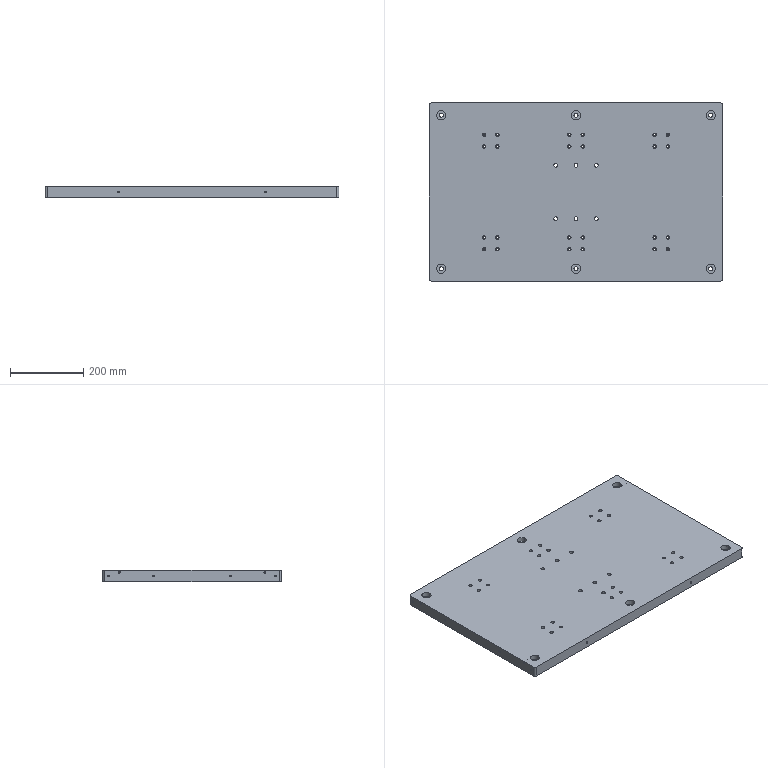NC program | Mastercam | posted with a generic post | part box 800 x 485 x 30 mm
Lines 1 to 982 of 7047:
%
O0000()
(MATERIAL - ALUMINUM MM - 2024)
( T20 | 20 FEM | H20 | XY STOCK TO LEAVE - .1 | Z STOCK TO LEAVE - .05 )
( T7 | 4 CHM | H7 )
( T1 | 11 DR | H1 )
( T15 | 5.5 DR | H15 )
( T14 | 10.5 DR | H14 )
( T5 | 5 FEM | H5 | XY STOCK TO LEAVE - -.01 | Z STOCK TO LEAVE - 0. )
( T9 | 10 FEM | H9 | XY STOCK TO LEAVE - .07 | Z STOCK TO LEAVE - .1 )
( T10 | 10 FEM | H10 | D10 | WEAR COMP | TOOL DIA. - 10. | XY STOCK TO LEAVE - -.02 | Z STOCK TO LEAVE - 0. )
( T18 | 5.1 DR | H18 )
N100 G21
N110 G0 G17 G40 G49 G80 G90
( ?X )
N120 T20 M6
N130 G0 G90 G54 X-415. Y252.6 A0. S5000 M3
N140 G43 H20 Z50. M8
N150 Z1.
N160 G1 Z-.998 F600.
N170 X-395. F4000.
N180 X395.
N190 X415.
N200 Z-1.997 F600.
N210 X395. F4000.
N220 X-395.
N230 X-415.
N240 Z-2.995 F600.
N250 X-395. F4000.
N260 X395.
N270 X415.
N280 Z-3.993 F600.
N290 X395. F4000.
N300 X-395.
N310 X-415.
N320 Z-4.992 F600.
N330 X-395. F4000.
N340 X395.
N350 X415.
N360 Z-5.99 F600.
N370 X395. F4000.
N380 X-395.
N390 X-415.
N400 Z-6.988 F600.
N410 X-395. F4000.
N420 X395.
N430 X415.
N440 Z-7.987 F600.
N450 X395. F4000.
N460 X-395.
N470 X-415.
N480 Z-8.985 F600.
N490 X-395. F4000.
N500 X395.
N510 X415.
N520 Z-9.983 F600.
N530 X395. F4000.
N540 X-395.
N550 X-415.
N560 Z-10.982 F600.
N570 X-395. F4000.
N580 X395.
N590 X415.
N600 Z-11.98 F600.
N610 X395. F4000.
N620 X-395.
N630 X-415.
N640 Z-12.978 F600.
N650 X-395. F4000.
N660 X395.
N670 X415.
N680 Z-13.977 F600.
N690 X395. F4000.
N700 X-395.
N710 X-415.
N720 Z-14.975 F600.
N730 X-395. F4000.
N740 X395.
N750 X415.
N760 Z-15.973 F600.
N770 X395. F4000.
N780 X-395.
N790 X-415.
N800 Z-16.972 F600.
N810 X-395. F4000.
N820 X395.
N830 X415.
N840 Z-17.97 F600.
N850 X395. F4000.
N860 X-395.
N870 X-415.
N880 Z-18.968 F600.
N890 X-395. F4000.
N900 X395.
N910 X415.
N920 Z-19.967 F600.
N930 X395. F4000.
N940 X-395.
N950 X-415.
N960 Z-20.965 F600.
N970 X-395. F4000.
N980 X395.
N990 X415.
N1000 Z-21.963 F600.
N1010 X395. F4000.
N1020 X-395.
N1030 X-415.
N1040 Z-22.962 F600.
N1050 X-395. F4000.
N1060 X395.
N1070 X415.
N1080 Z-23.96 F600.
N1090 X395. F4000.
N1100 X-395.
N1110 X-415.
N1120 Z-24.958 F600.
N1130 X-395. F4000.
N1140 X395.
N1150 X415.
N1160 Z-25.957 F600.
N1170 X395. F4000.
N1180 X-395.
N1190 X-415.
N1200 Z-26.955 F600.
N1210 X-395. F4000.
N1220 X395.
N1230 X415.
N1240 Z-27.953 F600.
N1250 X395. F4000.
N1260 X-395.
N1270 X-415.
N1280 Z-28.952 F600.
N1290 X-395. F4000.
N1300 X395.
N1310 X415.
N1320 Z-29.95 F600.
N1330 X395. F4000.
N1340 X-395.
N1350 X-415.
N1360 G0 Z50.
N1370 X415. Y-252.6
N1380 Z1.
N1390 G1 Z-.998 F600.
N1400 X395. F4000.
N1410 X-395.
N1420 X-415.
N1430 Z-1.997 F600.
N1440 X-395. F4000.
N1450 X395.
N1460 X415.
N1470 Z-2.995 F600.
N1480 X395. F4000.
N1490 X-395.
N1500 X-415.
N1510 Z-3.993 F600.
N1520 X-395. F4000.
N1530 X395.
N1540 X415.
N1550 Z-4.992 F600.
N1560 X395. F4000.
N1570 X-395.
N1580 X-415.
N1590 Z-5.99 F600.
N1600 X-395. F4000.
N1610 X395.
N1620 X415.
N1630 Z-6.988 F600.
N1640 X395. F4000.
N1650 X-395.
N1660 X-415.
N1670 Z-7.987 F600.
N1680 X-395. F4000.
N1690 X395.
N1700 X415.
N1710 Z-8.985 F600.
N1720 X395. F4000.
N1730 X-395.
N1740 X-415.
N1750 Z-9.983 F600.
N1760 X-395. F4000.
N1770 X395.
N1780 X415.
N1790 Z-10.982 F600.
N1800 X395. F4000.
N1810 X-395.
N1820 X-415.
N1830 Z-11.98 F600.
N1840 X-395. F4000.
N1850 X395.
N1860 X415.
N1870 Z-12.978 F600.
N1880 X395. F4000.
N1890 X-395.
N1900 X-415.
N1910 Z-13.977 F600.
N1920 X-395. F4000.
N1930 X395.
N1940 X415.
N1950 Z-14.975 F600.
N1960 X395. F4000.
N1970 X-395.
N1980 X-415.
N1990 Z-15.973 F600.
N2000 X-395. F4000.
N2010 X395.
N2020 X415.
N2030 Z-16.972 F600.
N2040 X395. F4000.
N2050 X-395.
N2060 X-415.
N2070 Z-17.97 F600.
N2080 X-395. F4000.
N2090 X395.
N2100 X415.
N2110 Z-18.968 F600.
N2120 X395. F4000.
N2130 X-395.
N2140 X-415.
N2150 Z-19.967 F600.
N2160 X-395. F4000.
N2170 X395.
N2180 X415.
N2190 Z-20.965 F600.
N2200 X395. F4000.
N2210 X-395.
N2220 X-415.
N2230 Z-21.963 F600.
N2240 X-395. F4000.
N2250 X395.
N2260 X415.
N2270 Z-22.962 F600.
N2280 X395. F4000.
N2290 X-395.
N2300 X-415.
N2310 Z-23.96 F600.
N2320 X-395. F4000.
N2330 X395.
N2340 X415.
N2350 Z-24.958 F600.
N2360 X395. F4000.
N2370 X-395.
N2380 X-415.
N2390 Z-25.957 F600.
N2400 X-395. F4000.
N2410 X395.
N2420 X415.
N2430 Z-26.955 F600.
N2440 X395. F4000.
N2450 X-395.
N2460 X-415.
N2470 Z-27.953 F600.
N2480 X-395. F4000.
N2490 X395.
N2500 X415.
N2510 Z-28.952 F600.
N2520 X395. F4000.
N2530 X-395.
N2540 X-415.
N2550 Z-29.95 F600.
N2560 X-395. F4000.
N2570 X395.
N2580 X415.
N2590 G0 Z50.
N2600 X-415. Y252.53
N2610 Z1.
N2620 G1 Z-29.95 F600.
N2630 X-395. F1000.
N2640 X395.
N2650 X415.
N2660 G0 Z50.
N2670 X-415. Y252.5
N2680 Z1.
N2690 G1 Z-29.95 F600.
N2700 X-395. F1000.
N2710 X395.
N2720 X415.
N2730 G0 Z50.
N2740 Y-252.53
N2750 Z1.
N2760 G1 Z-29.95 F600.
N2770 X395. F1000.
N2780 X-395.
N2790 X-415.
N2800 G0 Z50.
N2810 X415. Y-252.5
N2820 Z1.
N2830 G1 Z-29.95 F600.
N2840 X395. F1000.
N2850 X-395.
N2860 X-415.
N2870 G0 Z50.
N2880 M5
N2890 G91 G28 Z0. M9
N2900 A0.
N2910 M01
N2920 T7 M6
N2930 G0 G90 G17 G54 X-405. Y243.15 A0. S6500 M3
N2940 G43 H7 Z50. M8
N2950 Z1.
N2960 G1 Z-.75 F600.
N2970 X-395. F1000.
N2980 X395.
N2990 X405.
N3000 G0 Z50.
N3010 Y-243.15
N3020 Z1.
N3030 G1 Z-.75 F600.
N3040 X395. F1000.
N3050 X-395.
N3060 X-405.
N3070 G0 Z50.
N3080 M5
N3090 G91 G28 Z0. M9
N3100 A0.
N3110 M01
( CCL,CY )
M00
N3120 T20 M6
N3130 G0 G90 G17 G54 X-393. Y-256.6 A0. S5000 M3
N3140 G43 H20 Z50. M8
N3150 Z1.
N3160 G1 Z-.998 F600.
N3170 Y-254.6 F4000.
N3180 G3 X-395. Y-252.6 I-2. J0.
N3190 G2 X-410.1 Y-237.5 I0. J15.1
N3200 G1 Y237.5
N3210 G2 X-395. Y252.6 I15.1 J0.
N3220 G3 X-393. Y254.6 I0. J2.
N3230 G1 Y256.6
N3240 Z-1.997 F600.
N3250 Y254.6 F4000.
N3260 G2 X-395. Y252.6 I-2. J0.
N3270 G3 X-410.1 Y237.5 I0. J-15.1
N3280 G1 Y-237.5
N3290 G3 X-395. Y-252.6 I15.1 J0.
N3300 G2 X-393. Y-254.6 I0. J-2.
N3310 G1 Y-256.6
N3320 Z-2.995 F600.
N3330 Y-254.6 F4000.
N3340 G3 X-395. Y-252.6 I-2. J0.
N3350 G2 X-410.1 Y-237.5 I0. J15.1
N3360 G1 Y237.5
N3370 G2 X-395. Y252.6 I15.1 J0.
N3380 G3 X-393. Y254.6 I0. J2.
N3390 G1 Y256.6
N3400 Z-3.993 F600.
N3410 Y254.6 F4000.
N3420 G2 X-395. Y252.6 I-2. J0.
N3430 G3 X-410.1 Y237.5 I0. J-15.1
N3440 G1 Y-237.5
N3450 G3 X-395. Y-252.6 I15.1 J0.
N3460 G2 X-393. Y-254.6 I0. J-2.
N3470 G1 Y-256.6
N3480 Z-4.992 F600.
N3490 Y-254.6 F4000.
N3500 G3 X-395. Y-252.6 I-2. J0.
N3510 G2 X-410.1 Y-237.5 I0. J15.1
N3520 G1 Y237.5
N3530 G2 X-395. Y252.6 I15.1 J0.
N3540 G3 X-393. Y254.6 I0. J2.
N3550 G1 Y256.6
N3560 Z-5.99 F600.
N3570 Y254.6 F4000.
N3580 G2 X-395. Y252.6 I-2. J0.
N3590 G3 X-410.1 Y237.5 I0. J-15.1
N3600 G1 Y-237.5
N3610 G3 X-395. Y-252.6 I15.1 J0.
N3620 G2 X-393. Y-254.6 I0. J-2.
N3630 G1 Y-256.6
N3640 Z-6.988 F600.
N3650 Y-254.6 F4000.
N3660 G3 X-395. Y-252.6 I-2. J0.
N3670 G2 X-410.1 Y-237.5 I0. J15.1
N3680 G1 Y237.5
N3690 G2 X-395. Y252.6 I15.1 J0.
N3700 G3 X-393. Y254.6 I0. J2.
N3710 G1 Y256.6
N3720 Z-7.987 F600.
N3730 Y254.6 F4000.
N3740 G2 X-395. Y252.6 I-2. J0.
N3750 G3 X-410.1 Y237.5 I0. J-15.1
N3760 G1 Y-237.5
N3770 G3 X-395. Y-252.6 I15.1 J0.
N3780 G2 X-393. Y-254.6 I0. J-2.
N3790 G1 Y-256.6
N3800 Z-8.985 F600.
N3810 Y-254.6 F4000.
N3820 G3 X-395. Y-252.6 I-2. J0.
N3830 G2 X-410.1 Y-237.5 I0. J15.1
N3840 G1 Y237.5
N3850 G2 X-395. Y252.6 I15.1 J0.
N3860 G3 X-393. Y254.6 I0. J2.
N3870 G1 Y256.6
N3880 Z-9.983 F600.
N3890 Y254.6 F4000.
N3900 G2 X-395. Y252.6 I-2. J0.
N3910 G3 X-410.1 Y237.5 I0. J-15.1
N3920 G1 Y-237.5
N3930 G3 X-395. Y-252.6 I15.1 J0.
N3940 G2 X-393. Y-254.6 I0. J-2.
N3950 G1 Y-256.6
N3960 Z-10.982 F600.
N3970 Y-254.6 F4000.
N3980 G3 X-395. Y-252.6 I-2. J0.
N3990 G2 X-410.1 Y-237.5 I0. J15.1
N4000 G1 Y237.5
N4010 G2 X-395. Y252.6 I15.1 J0.
N4020 G3 X-393. Y254.6 I0. J2.
N4030 G1 Y256.6
N4040 Z-11.98 F600.
N4050 Y254.6 F4000.
N4060 G2 X-395. Y252.6 I-2. J0.
N4070 G3 X-410.1 Y237.5 I0. J-15.1
N4080 G1 Y-237.5
N4090 G3 X-395. Y-252.6 I15.1 J0.
N4100 G2 X-393. Y-254.6 I0. J-2.
N4110 G1 Y-256.6
N4120 Z-12.978 F600.
N4130 Y-254.6 F4000.
N4140 G3 X-395. Y-252.6 I-2. J0.
N4150 G2 X-410.1 Y-237.5 I0. J15.1
N4160 G1 Y237.5
N4170 G2 X-395. Y252.6 I15.1 J0.
N4180 G3 X-393. Y254.6 I0. J2.
N4190 G1 Y256.6
N4200 Z-13.977 F600.
N4210 Y254.6 F4000.
N4220 G2 X-395. Y252.6 I-2. J0.
N4230 G3 X-410.1 Y237.5 I0. J-15.1
N4240 G1 Y-237.5
N4250 G3 X-395. Y-252.6 I15.1 J0.
N4260 G2 X-393. Y-254.6 I0. J-2.
N4270 G1 Y-256.6
N4280 Z-14.975 F600.
N4290 Y-254.6 F4000.
N4300 G3 X-395. Y-252.6 I-2. J0.
N4310 G2 X-410.1 Y-237.5 I0. J15.1
N4320 G1 Y237.5
N4330 G2 X-395. Y252.6 I15.1 J0.
N4340 G3 X-393. Y254.6 I0. J2.
N4350 G1 Y256.6
N4360 Z-15.973 F600.
N4370 Y254.6 F4000.
N4380 G2 X-395. Y252.6 I-2. J0.
N4390 G3 X-410.1 Y237.5 I0. J-15.1
N4400 G1 Y-237.5
N4410 G3 X-395. Y-252.6 I15.1 J0.
N4420 G2 X-393. Y-254.6 I0. J-2.
N4430 G1 Y-256.6
N4440 Z-16.972 F600.
N4450 Y-254.6 F4000.
N4460 G3 X-395. Y-252.6 I-2. J0.
N4470 G2 X-410.1 Y-237.5 I0. J15.1
N4480 G1 Y237.5
N4490 G2 X-395. Y252.6 I15.1 J0.
N4500 G3 X-393. Y254.6 I0. J2.
N4510 G1 Y256.6
N4520 Z-17.97 F600.
N4530 Y254.6 F4000.
N4540 G2 X-395. Y252.6 I-2. J0.
N4550 G3 X-410.1 Y237.5 I0. J-15.1
N4560 G1 Y-237.5
N4570 G3 X-395. Y-252.6 I15.1 J0.
N4580 G2 X-393. Y-254.6 I0. J-2.
N4590 G1 Y-256.6
N4600 Z-18.968 F600.
N4610 Y-254.6 F4000.
N4620 G3 X-395. Y-252.6 I-2. J0.
N4630 G2 X-410.1 Y-237.5 I0. J15.1
N4640 G1 Y237.5
N4650 G2 X-395. Y252.6 I15.1 J0.
N4660 G3 X-393. Y254.6 I0. J2.
N4670 G1 Y256.6
N4680 Z-19.967 F600.
N4690 Y254.6 F4000.
N4700 G2 X-395. Y252.6 I-2. J0.
N4710 G3 X-410.1 Y237.5 I0. J-15.1
N4720 G1 Y-237.5
N4730 G3 X-395. Y-252.6 I15.1 J0.
N4740 G2 X-393. Y-254.6 I0. J-2.
N4750 G1 Y-256.6
N4760 Z-20.965 F600.
N4770 Y-254.6 F4000.
N4780 G3 X-395. Y-252.6 I-2. J0.
N4790 G2 X-410.1 Y-237.5 I0. J15.1
N4800 G1 Y237.5
N4810 G2 X-395. Y252.6 I15.1 J0.
N4820 G3 X-393. Y254.6 I0. J2.
N4830 G1 Y256.6
N4840 Z-21.963 F600.
N4850 Y254.6 F4000.
N4860 G2 X-395. Y252.6 I-2. J0.
N4870 G3 X-410.1 Y237.5 I0. J-15.1
N4880 G1 Y-237.5
N4890 G3 X-395. Y-252.6 I15.1 J0.
N4900 G2 X-393. Y-254.6 I0. J-2.
N4910 G1 Y-256.6
N4920 Z-22.962 F600.
N4930 Y-254.6 F4000.
N4940 G3 X-395. Y-252.6 I-2. J0.
N4950 G2 X-410.1 Y-237.5 I0. J15.1
N4960 G1 Y237.5
N4970 G2 X-395. Y252.6 I15.1 J0.
N4980 G3 X-393. Y254.6 I0. J2.
N4990 G1 Y256.6
N5000 Z-23.96 F600.
N5010 Y254.6 F4000.
N5020 G2 X-395. Y252.6 I-2. J0.
N5030 G3 X-410.1 Y237.5 I0. J-15.1
N5040 G1 Y-237.5
N5050 G3 X-395. Y-252.6 I15.1 J0.
N5060 G2 X-393. Y-254.6 I0. J-2.
N5070 G1 Y-256.6
N5080 Z-24.958 F600.
N5090 Y-254.6 F4000.
N5100 G3 X-395. Y-252.6 I-2. J0.
N5110 G2 X-410.1 Y-237.5 I0. J15.1
N5120 G1 Y237.5
N5130 G2 X-395. Y252.6 I15.1 J0.
N5140 G3 X-393. Y254.6 I0. J2.
N5150 G1 Y256.6
N5160 Z-25.957 F600.
N5170 Y254.6 F4000.
N5180 G2 X-395. Y252.6 I-2. J0.
N5190 G3 X-410.1 Y237.5 I0. J-15.1
N5200 G1 Y-237.5
N5210 G3 X-395. Y-252.6 I15.1 J0.
N5220 G2 X-393. Y-254.6 I0. J-2.
N5230 G1 Y-256.6
N5240 Z-26.955 F600.
N5250 Y-254.6 F4000.
N5260 G3 X-395. Y-252.6 I-2. J0.
N5270 G2 X-410.1 Y-237.5 I0. J15.1
N5280 G1 Y237.5
N5290 G2 X-395. Y252.6 I15.1 J0.
N5300 G3 X-393. Y254.6 I0. J2.
N5310 G1 Y256.6
N5320 Z-27.953 F600.
N5330 Y254.6 F4000.
N5340 G2 X-395. Y252.6 I-2. J0.
N5350 G3 X-410.1 Y237.5 I0. J-15.1
N5360 G1 Y-237.5
N5370 G3 X-395. Y-252.6 I15.1 J0.
N5380 G2 X-393. Y-254.6 I0. J-2.
N5390 G1 Y-256.6
N5400 Z-28.952 F600.
N5410 Y-254.6 F4000.
N5420 G3 X-395. Y-252.6 I-2. J0.
N5430 G2 X-410.1 Y-237.5 I0. J15.1
N5440 G1 Y237.5
N5450 G2 X-395. Y252.6 I15.1 J0.
N5460 G3 X-393. Y254.6 I0. J2.
N5470 G1 Y256.6
N5480 Z-29.95 F600.
N5490 Y254.6 F4000.
N5500 G2 X-395. Y252.6 I-2. J0.
N5510 G3 X-410.1 Y237.5 I0. J-15.1
N5520 G1 Y-237.5
N5530 G3 X-395. Y-252.6 I15.1 J0.
N5540 G2 X-393. Y-254.6 I0. J-2.
N5550 G1 Y-256.6
N5560 G0 Z50.
N5570 X393. Y256.6
N5580 Z1.
N5590 G1 Z-.998 F600.
N5600 Y254.6 F4000.
N5610 G3 X395. Y252.6 I2. J0.
N5620 G2 X410.1 Y237.5 I0. J-15.1
N5630 G1 Y-237.5
N5640 G2 X395. Y-252.6 I-15.1 J0.
N5650 G3 X393. Y-254.6 I0. J-2.
N5660 G1 Y-256.6
N5670 Z-1.997 F600.
N5680 Y-254.6 F4000.
N5690 G2 X395. Y-252.6 I2. J0.
N5700 G3 X410.1 Y-237.5 I0. J15.1
N5710 G1 Y237.5
N5720 G3 X395. Y252.6 I-15.1 J0.
N5730 G2 X393. Y254.6 I0. J2.
N5740 G1 Y256.6
N5750 Z-2.995 F600.
N5760 Y254.6 F4000.
N5770 G3 X395. Y252.6 I2. J0.
N5780 G2 X410.1 Y237.5 I0. J-15.1
N5790 G1 Y-237.5
N5800 G2 X395. Y-252.6 I-15.1 J0.
N5810 G3 X393. Y-254.6 I0. J-2.
N5820 G1 Y-256.6
N5830 Z-3.993 F600.
N5840 Y-254.6 F4000.
N5850 G2 X395. Y-252.6 I2. J0.
N5860 G3 X410.1 Y-237.5 I0. J15.1
N5870 G1 Y237.5
N5880 G3 X395. Y252.6 I-15.1 J0.
N5890 G2 X393. Y254.6 I0. J2.
N5900 G1 Y256.6
N5910 Z-4.992 F600.
N5920 Y254.6 F4000.
N5930 G3 X395. Y252.6 I2. J0.
N5940 G2 X410.1 Y237.5 I0. J-15.1
N5950 G1 Y-237.5
N5960 G2 X395. Y-252.6 I-15.1 J0.
N5970 G3 X393. Y-254.6 I0. J-2.
N5980 G1 Y-256.6
N5990 Z-5.99 F600.
N6000 Y-254.6 F4000.
N6010 G2 X395. Y-252.6 I2. J0.
N6020 G3 X410.1 Y-237.5 I0. J15.1
N6030 G1 Y237.5
N6040 G3 X395. Y252.6 I-15.1 J0.
N6050 G2 X393. Y254.6 I0. J2.
N6060 G1 Y256.6
N6070 Z-6.988 F600.
N6080 Y254.6 F4000.
N6090 G3 X395. Y252.6 I2. J0.
N6100 G2 X410.1 Y237.5 I0. J-15.1
N6110 G1 Y-237.5
N6120 G2 X395. Y-252.6 I-15.1 J0.
N6130 G3 X393. Y-254.6 I0. J-2.
N6140 G1 Y-256.6
N6150 Z-7.987 F600.
N6160 Y-254.6 F4000.
N6170 G2 X395. Y-252.6 I2. J0.
N6180 G3 X410.1 Y-237.5 I0. J15.1
N6190 G1 Y237.5
N6200 G3 X395. Y252.6 I-15.1 J0.
N6210 G2 X393. Y254.6 I0. J2.
N6220 G1 Y256.6
N6230 Z-8.985 F600.
N6240 Y254.6 F4000.
N6250 G3 X395. Y252.6 I2. J0.
N6260 G2 X410.1 Y237.5 I0. J-15.1
N6270 G1 Y-237.5
N6280 G2 X395. Y-252.6 I-15.1 J0.
N6290 G3 X393. Y-254.6 I0. J-2.
N6300 G1 Y-256.6
N6310 Z-9.983 F600.
N6320 Y-254.6 F4000.
N6330 G2 X395. Y-252.6 I2. J0.
N6340 G3 X410.1 Y-237.5 I0. J15.1
N6350 G1 Y237.5
N6360 G3 X395. Y252.6 I-15.1 J0.
N6370 G2 X393. Y254.6 I0. J2.
N6380 G1 Y256.6
N6390 Z-10.982 F600.
N6400 Y254.6 F4000.
N6410 G3 X395. Y252.6 I2. J0.
N6420 G2 X410.1 Y237.5 I0. J-15.1
N6430 G1 Y-237.5
N6440 G2 X395. Y-252.6 I-15.1 J0.
N6450 G3 X393. Y-254.6 I0. J-2.
N6460 G1 Y-256.6
N6470 Z-11.98 F600.
N6480 Y-254.6 F4000.
N6490 G2 X395. Y-252.6 I2. J0.
N6500 G3 X410.1 Y-237.5 I0. J15.1
N6510 G1 Y237.5
N6520 G3 X395. Y252.6 I-15.1 J0.
N6530 G2 X393. Y254.6 I0. J2.
N6540 G1 Y256.6
N6550 Z-12.978 F600.
N6560 Y254.6 F4000.
N6570 G3 X395. Y252.6 I2. J0.
N6580 G2 X410.1 Y237.5 I0. J-15.1
N6590 G1 Y-237.5
N6600 G2 X395. Y-252.6 I-15.1 J0.
N6610 G3 X393. Y-254.6 I0. J-2.
N6620 G1 Y-256.6
N6630 Z-13.977 F600.
N6640 Y-254.6 F4000.
N6650 G2 X395. Y-252.6 I2. J0.
N6660 G3 X410.1 Y-237.5 I0. J15.1
N6670 G1 Y237.5
N6680 G3 X395. Y252.6 I-15.1 J0.
N6690 G2 X393. Y254.6 I0. J2.
N6700 G1 Y256.6
N6710 Z-14.975 F600.
N6720 Y254.6 F4000.
N6730 G3 X395. Y252.6 I2. J0.
N6740 G2 X410.1 Y237.5 I0. J-15.1
N6750 G1 Y-237.5
N6760 G2 X395. Y-252.6 I-15.1 J0.
N6770 G3 X393. Y-254.6 I0. J-2.
N6780 G1 Y-256.6
N6790 Z-15.973 F600.
N6800 Y-254.6 F4000.
N6810 G2 X395. Y-252.6 I2. J0.
N6820 G3 X410.1 Y-237.5 I0. J15.1
N6830 G1 Y237.5
N6840 G3 X395. Y252.6 I-15.1 J0.
N6850 G2 X393. Y254.6 I0. J2.
N6860 G1 Y256.6
N6870 Z-16.972 F600.
N6880 Y254.6 F4000.
N6890 G3 X395. Y252.6 I2. J0.
N6900 G2 X410.1 Y237.5 I0. J-15.1
N6910 G1 Y-237.5
N6920 G2 X395. Y-252.6 I-15.1 J0.
N6930 G3 X393. Y-254.6 I0. J-2.
N6940 G1 Y-256.6
N6950 Z-17.97 F600.
N6960 Y-254.6 F4000.
N6970 G2 X395. Y-252.6 I2. J0.
N6980 G3 X410.1 Y-237.5 I0. J15.1
N6990 G1 Y237.5
N7000 G3 X395. Y252.6 I-15.1 J0.
N7010 G2 X393. Y254.6 I0. J2.
N7020 G1 Y256.6
N7030 Z-18.968 F600.
N7040 Y254.6 F4000.
N7050 G3 X395. Y252.6 I2. J0.
N7060 G2 X410.1 Y237.5 I0. J-15.1
N7070 G1 Y-237.5
N7080 G2 X395. Y-252.6 I-15.1 J0.
N7090 G3 X393. Y-254.6 I0. J-2.
N7100 G1 Y-256.6
N7110 Z-19.967 F600.
N7120 Y-254.6 F4000.
N7130 G2 X395. Y-252.6 I2. J0.
N7140 G3 X410.1 Y-237.5 I0. J15.1
N7150 G1 Y237.5
N7160 G3 X395. Y252.6 I-15.1 J0.
N7170 G2 X393. Y254.6 I0. J2.
N7180 G1 Y256.6
N7190 Z-20.965 F600.
N7200 Y254.6 F4000.
N7210 G3 X395. Y252.6 I2. J0.
N7220 G2 X410.1 Y237.5 I0. J-15.1
N7230 G1 Y-237.5
N7240 G2 X395. Y-252.6 I-15.1 J0.
N7250 G3 X393. Y-254.6 I0. J-2.
N7260 G1 Y-256.6
N7270 Z-21.963 F600.
N7280 Y-254.6 F4000.
N7290 G2 X395. Y-252.6 I2. J0.
N7300 G3 X410.1 Y-237.5 I0. J15.1
N7310 G1 Y237.5
N7320 G3 X395. Y252.6 I-15.1 J0.
N7330 G2 X393. Y254.6 I0. J2.
N7340 G1 Y256.6
N7350 Z-22.962 F600.
N7360 Y254.6 F4000.
N7370 G3 X395. Y252.6 I2. J0.
N7380 G2 X410.1 Y237.5 I0. J-15.1
N7390 G1 Y-237.5
N7400 G2 X395. Y-252.6 I-15.1 J0.
N7410 G3 X393. Y-254.6 I0. J-2.
N7420 G1 Y-256.6
N7430 Z-23.96 F600.
N7440 Y-254.6 F4000.
N7450 G2 X395. Y-252.6 I2. J0.
N7460 G3 X410.1 Y-237.5 I0. J15.1
N7470 G1 Y237.5
N7480 G3 X395. Y252.6 I-15.1 J0.
N7490 G2 X393. Y254.6 I0. J2.
N7500 G1 Y256.6
N7510 Z-24.958 F600.
N7520 Y254.6 F4000.
N7530 G3 X395. Y252.6 I2. J0.
N7540 G2 X410.1 Y237.5 I0. J-15.1
N7550 G1 Y-237.5
N7560 G2 X395. Y-252.6 I-15.1 J0.
N7570 G3 X393. Y-254.6 I0. J-2.
N7580 G1 Y-256.6
N7590 Z-25.957 F600.
N7600 Y-254.6 F4000.
N7610 G2 X395. Y-252.6 I2. J0.
N7620 G3 X410.1 Y-237.5 I0. J15.1
N7630 G1 Y237.5
N7640 G3 X395. Y252.6 I-15.1 J0.
N7650 G2 X393. Y254.6 I0. J2.
N7660 G1 Y256.6
N7670 Z-26.955 F600.
N7680 Y254.6 F4000.
N7690 G3 X395. Y252.6 I2. J0.
N7700 G2 X410.1 Y237.5 I0. J-15.1
N7710 G1 Y-237.5
N7720 G2 X395. Y-252.6 I-15.1 J0.
N7730 G3 X393. Y-254.6 I0. J-2.
N7740 G1 Y-256.6
N7750 Z-27.953 F600.
N7760 Y-254.6 F4000.
N7770 G2 X395. Y-252.6 I2. J0.
N7780 G3 X410.1 Y-237.5 I0. J15.1
N7790 G1 Y237.5
N7800 G3 X395. Y252.6 I-15.1 J0.
N7810 G2 X393. Y254.6 I0. J2.
N7820 G1 Y256.6
N7830 Z-28.952 F600.
N7840 Y254.6 F4000.
N7850 G3 X395. Y252.6 I2. J0.
N7860 G2 X410.1 Y237.5 I0. J-15.1
N7870 G1 Y-237.5
N7880 G2 X395. Y-252.6 I-15.1 J0.
N7890 G3 X393. Y-254.6 I0. J-2.
N7900 G1 Y-256.6
N7910 Z-29.95 F600.
N7920 Y-254.6 F4000.
N7930 G2 X395. Y-252.6 I2. J0.
N7940 G3 X410.1 Y-237.5 I0. J15.1
N7950 G1 Y237.5
N7960 G3 X395. Y252.6 I-15.1 J0.
N7970 G2 X393. Y254.6 I0. J2.
N7980 G1 Y256.6
N7990 G0 Z50.
N8000 X-393. Y-256.53
N8010 Z1.
N8020 G1 Z-29.95 F600.
N8030 Y-254.53 F1000.
N8040 G3 X-395. Y-252.53 I-2. J0.
N8050 G2 X-410.03 Y-237.5 I0. J15.03
N8060 G1 Y237.5
N8070 G2 X-395. Y252.53 I15.03 J0.
N8080 G3 X-393. Y254.53 I0. J2.
N8090 G1 Y256.53
N8100 G0 Z50.
N8110 Y-256.5
N8120 Z1.
N8130 G1 Z-29.95 F600.
N8140 Y-254.5 F1000.
N8150 G3 X-395. Y-252.5 I-2. J0.
N8160 G2 X-410. Y-237.5 I0. J15.
N8170 G1 Y237.5
N8180 G2 X-395. Y252.5 I15. J0.
N8190 G3 X-393. Y254.5 I0. J2.
N8200 G1 Y256.5
N8210 G0 Z50.
N8220 X393. Y256.53
N8230 Z1.
N8240 G1 Z-29.95 F600.
N8250 Y254.53 F1000.
N8260 G3 X395. Y252.53 I2. J0.
N8270 G2 X410.03 Y237.5 I0. J-15.03
N8280 G1 Y-237.5
N8290 G2 X395. Y-252.53 I-15.03 J0.
N8300 G3 X393. Y-254.53 I0. J-2.
N8310 G1 Y-256.53
N8320 G0 Z50.
N8330 Y256.5
N8340 Z1.
N8350 G1 Z-29.95 F600.
N8360 Y254.5 F1000.
N8370 G3 X395. Y252.5 I2. J0.
N8380 G2 X410. Y237.5 I0. J-15.
N8390 G1 Y-237.5
N8400 G2 X395. Y-252.5 I-15. J0.
N8410 G3 X393. Y-254.5 I0. J-2.
N8420 G1 Y-256.5
N8430 G0 Z50.
N8440 M5
N8450 G91 G28 Z0. M9
N8460 A0.
N8470 M01
N8480 T7 M6
N8490 G0 G90 G17 G54 X-394.6 Y-243.95 A0. S6500 M3
N8500 G43 H7 Z50. M8
N8510 Z1.
N8520 G1 Z-.75 F600.
N8530 Y-243.55 F1000.
N8540 G3 X-395. Y-243.15 I-.4 J0.
N8550 G2 X-400.65 Y-237.5 I0. J5.65
N8560 G1 Y237.5
N8570 G2 X-395. Y243.15 I5.65 J0.
N8580 G3 X-394.6 Y243.55 I0. J.4
N8590 G1 Y243.95
N8600 G0 Z50.
N8610 X394.6
N8620 Z1.
N8630 G1 Z-.75 F600.
N8640 Y243.55 F1000.
N8650 G3 X395. Y243.15 I.4 J0.
N8660 G2 X400.65 Y237.5 I0. J-5.65
N8670 G1 Y-237.5
N8680 G2 X395. Y-243.15 I-5.65 J0.
N8690 G3 X394.6 Y-243.55 I0. J-.4
N8700 G1 Y-243.95
N8710 G0 Z50.
( X+CL )
M00
N8720 S6000 M3
N8730 X367. Y-209.
N8740 G98 G81 Z-.7 R1. F200.
N8750 X250. Y-156.
N8760 Y-124.
N8770 X214.
N8780 Y-156.
N8790 X0. Y-209.
N8800 X-214. Y-156.
N8810 Y-124.
N8820 X-250.
N8830 Y-156.
N8840 X-367. Y-209.
N8850 Y209.
N8860 X-250. Y156.
N8870 Y124.
N8880 X-214.
N8890 Y156.
N8900 X-18. Y124.
N8910 Y156.
N8920 X0. Y209.
N8930 X18. Y156.
N8940 Y124.
N8950 X55. Y72.5
N8960 X0.
N8970 X-55.
N8980 Y-72.5
N8990 X-18. Y-124.
N9000 Y-156.
N9010 X18.
N9020 Y-124.
N9030 X0. Y-72.5
N9040 X55.
N9050 X214. Y124.
N9060 Y156.
N9070 X250. Y124.
N9080 Y156.
N9090 X367. Y209.
N9100 G80
N9110 M5
N9120 G91 G0 G28 Z0. M9
N9130 A0.
N9140 M01
N9150 T1 M6
N9160 G0 G90 G17 G54 X367. Y-209. A0. S800 M3
N9170 G43 H1 Z50. M8
N9180 G98 G83 Z-29.8 R1. Q2. F80.
N9190 X0.
N9200 X-367.
N9210 Y209.
N9220 X0.
N9230 X367.
N9240 G80
N9250 M5
N9260 G91 G0 G28 Z0. M9
N9270 A0.
N9280 M01
N9290 T15 M6
N9300 G0 G90 G17 G54 X250. Y-156. A0. S1200 M3
N9310 G43 H15 Z50. M8
N9320 G98 G83 Z-29.8 R1. Q2. F120.
N9330 Y-124.
N9340 X214.
N9350 Y-156.
N9360 X18.
N9370 Y-124.
N9380 X-18.
N9390 Y-156.
N9400 X-214. Y-124.
N9410 Y-156.
N9420 X-250.
N9430 Y-124.
N9440 Y124.
N9450 Y156.
N9460 X-214.
N9470 Y124.
N9480 X-18.
N9490 Y156.
N9500 X18.
N9510 Y124.
N9520 X214.
N9530 Y156.
N9540 X250.
N9550 Y124.
N9560 G80
N9570 M5
N9580 G91 G0 G28 Z0. M9
N9590 A0.
N9600 M01
N9610 T14 M6
N9620 G0 G90 G17 G54 X55. Y-72.5 A0. S800 M3
N9630 G43 H14 Z50. M8
N9640 G98 G83 Z-29.8 R1. Q2. F100.
N9650 X0.
N9660 X-55.
N9670 Y72.5
N9680 X0.
N9690 X55.
N9700 G80
N9710 M5
N9720 G91 G0 G28 Z0. M9
N9730 A0.
N9740 M01